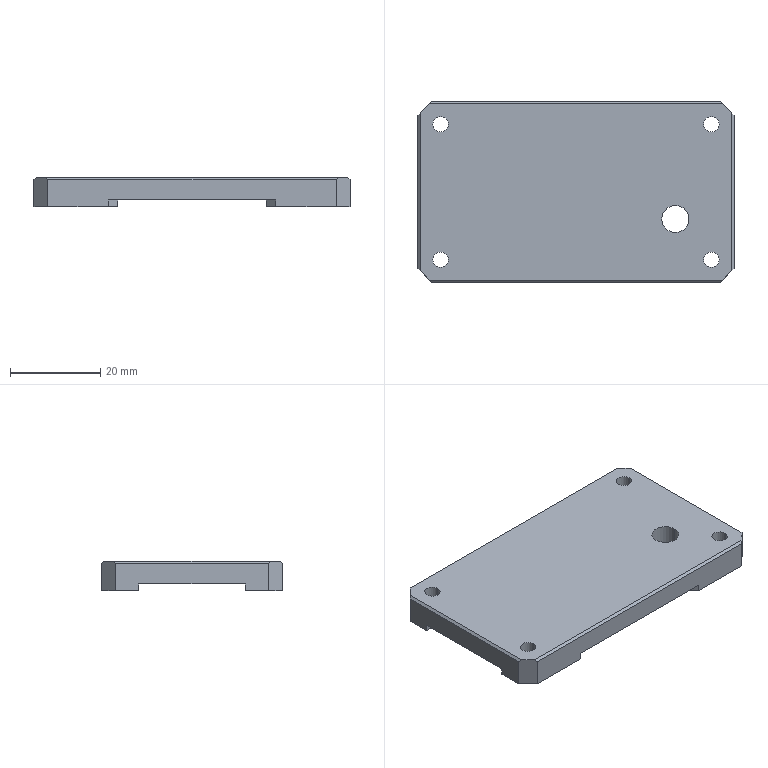Part | STEP file | 11-FG-Z00311 | 1 solid | 68 faces | box 70 x 40 x 6.5 mm | volume 14188 mm3 | plane 46 | cylinder 22 | commonest cylinder face diameters 3.4 x8 6.5 x8 2 x4 6 x2